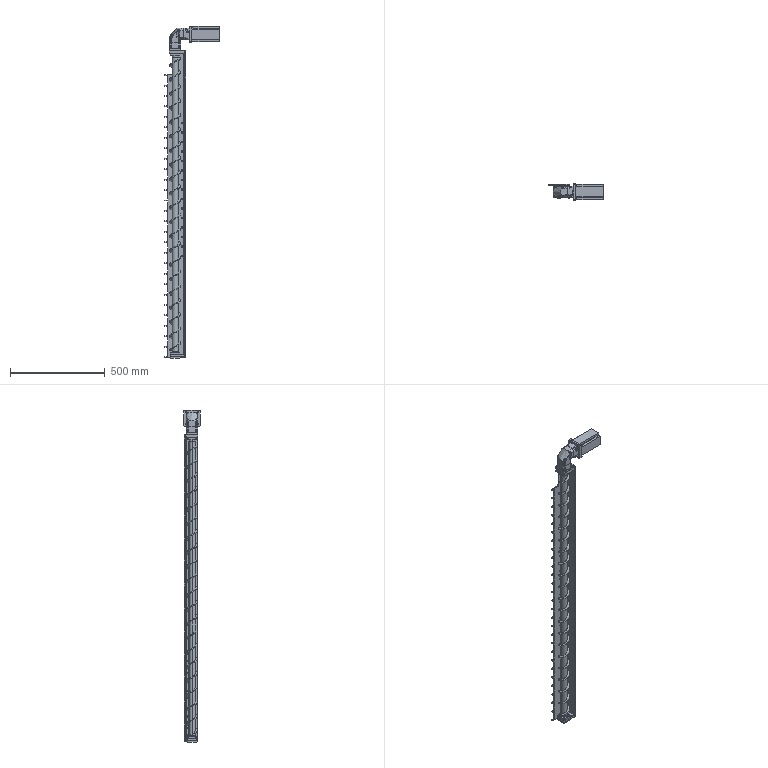Part | SolidWorks | features InContextFeatHolder 8, CompositeCurve 2 | 27 solids | 1302 faces | box 286 x 85 x 1747 mm | volume 3475124 mm3 | cylinder 626 | plane 457 | cone 126 | spline 53 | torus 40 | commonest cylinder face diameters 6.8 x120 4.2 x60 5.5 x56 5.8 x49 10 x27 69 x26